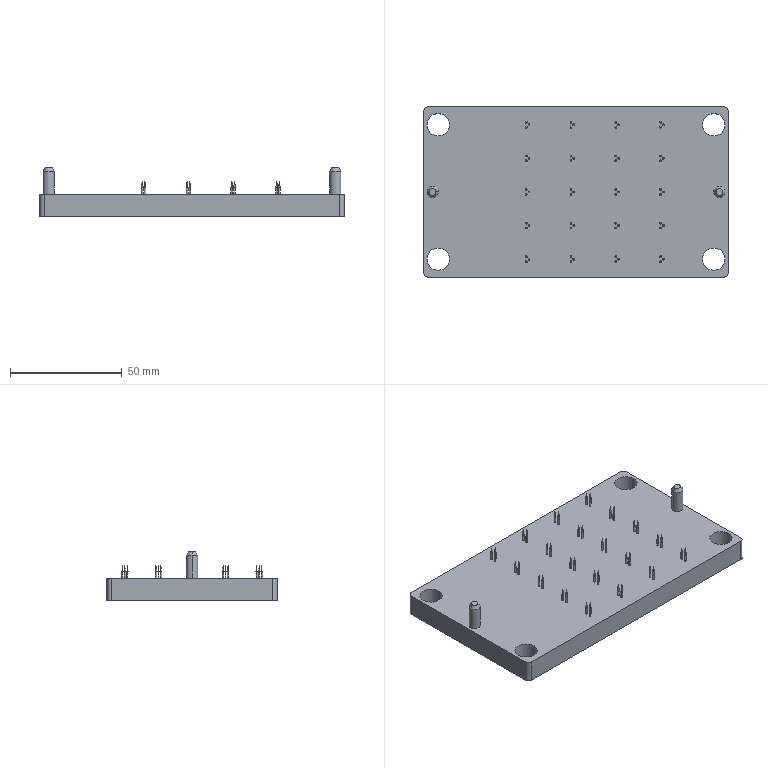Part | STEP file | FBDS-CS-029 | 1 solid | 268 faces | box 136 x 76 x 22 mm | volume 100751 mm3 | cylinder 136 | cone 124 | plane 8 | commonest cylinder face diameters 0.8 x120 10 x8 4 x4 5 x4